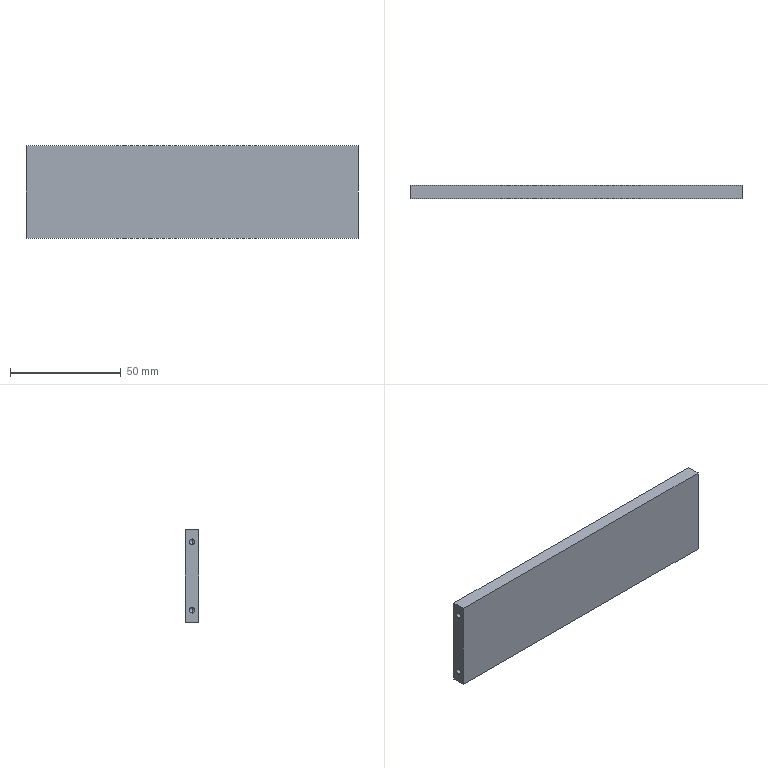Part | SolidWorks | features Cut 2, HoleWzd 2, Extrusion 1 | 1 solid | 22 faces | box 150 x 6 x 42 mm | volume 37648 mm3 | cone 8 | cylinder 8 | plane 6 | commonest cylinder face diameters 2.5 x8
STEP:
#1=CARTESIAN_POINT('',(-66.749,3.,-15.5));
#2=VERTEX_POINT('',#1);
#3=CARTESIAN_POINT('',(-67.5,3.,-14.25));
#4=VERTEX_POINT('',#3);
#5=CARTESIAN_POINT('',(-67.5,3.,-14.25));
#6=DIRECTION('',(-0.515,0.,0.8572));
#7=VECTOR('',#6,1000.);
#8=LINE('',#5,#7);
#9=EDGE_CURVE('',#2,#4,#8,.T.);
#10=ORIENTED_EDGE('',*,*,#9,.F.);
#11=CARTESIAN_POINT('',(-67.5,3.,-16.75));
#12=VERTEX_POINT('',#11);
#13=CARTESIAN_POINT('',(-67.5,3.,-16.75));
#14=DIRECTION('',(-0.515,0.,-0.8572));
#15=VECTOR('',#14,1000.);
#16=LINE('',#13,#15);
#17=EDGE_CURVE('',#2,#12,#16,.T.);
#18=ORIENTED_EDGE('',*,*,#17,.T.);
#19=CARTESIAN_POINT('',(-67.5,3.,-15.5));
#20=DIRECTION('',(-1.,0.,0.));
#21=DIRECTION('',(0.,0.,1.));
#22=AXIS2_PLACEMENT_3D('',#19,#20,#21);
#23=CIRCLE('',#22,1.25);
#24=EDGE_CURVE('',#12,#4,#23,.T.);
#25=ORIENTED_EDGE('',*,*,#24,.T.);
#26=EDGE_LOOP('',(#10,#18,#25));
#27=FACE_OUTER_BOUND('',#26,.T.);
#28=CARTESIAN_POINT('',(-67.5,3.,-15.5));
#29=DIRECTION('',(-1.,0.,0.));
#30=DIRECTION('',(0.,0.,1.));
#31=AXIS2_PLACEMENT_3D('',#28,#29,#30);
#32=CONICAL_SURFACE('',#31,1.25,1.03);
#33=ADVANCED_FACE('',(#27),#32,.F.);
#34=CARTESIAN_POINT('',(-66.749,3.,15.5));
#35=VERTEX_POINT('',#34);
#36=CARTESIAN_POINT('',(-67.5,3.,16.75));
#37=VERTEX_POINT('',#36);
#38=CARTESIAN_POINT('',(-67.5,3.,16.75));
#39=DIRECTION('',(-0.515,0.,0.8572));
#40=VECTOR('',#39,1000.);
#41=LINE('',#38,#40);
#42=EDGE_CURVE('',#35,#37,#41,.T.);
#43=ORIENTED_EDGE('',*,*,#42,.F.);
#44=CARTESIAN_POINT('',(-67.5,3.,14.25));
#45=VERTEX_POINT('',#44);
#46=CARTESIAN_POINT('',(-67.5,3.,14.25));
#47=DIRECTION('',(-0.515,0.,-0.8572));
#48=VECTOR('',#47,1000.);
#49=LINE('',#46,#48);
#50=EDGE_CURVE('',#35,#45,#49,.T.);
#51=ORIENTED_EDGE('',*,*,#50,.T.);
#52=CARTESIAN_POINT('',(-67.5,3.,15.5));
#53=DIRECTION('',(-1.,0.,0.));
#54=DIRECTION('',(0.,0.,1.));
#55=AXIS2_PLACEMENT_3D('',#52,#53,#54);
#56=CIRCLE('',#55,1.25);
#57=EDGE_CURVE('',#45,#37,#56,.T.);
#58=ORIENTED_EDGE('',*,*,#57,.T.);
#59=EDGE_LOOP('',(#43,#51,#58));
#60=FACE_OUTER_BOUND('',#59,.T.);
#61=CARTESIAN_POINT('',(-67.5,3.,15.5));
#62=DIRECTION('',(-1.,0.,0.));
#63=DIRECTION('',(0.,0.,1.));
#64=AXIS2_PLACEMENT_3D('',#61,#62,#63);
#65=CONICAL_SURFACE('',#64,1.25,1.03);
#66=ADVANCED_FACE('',(#60),#65,.F.);
#67=CARTESIAN_POINT('',(66.749,3.,15.5));
#68=VERTEX_POINT('',#67);
#69=CARTESIAN_POINT('',(67.5,3.,14.25));
#70=VERTEX_POINT('',#69);
#71=CARTESIAN_POINT('',(67.5,3.,14.25));
#72=DIRECTION('',(0.515,0.,-0.8572));
#73=VECTOR('',#72,1000.);
#74=LINE('',#71,#73);
#75=EDGE_CURVE('',#68,#70,#74,.T.);
#76=ORIENTED_EDGE('',*,*,#75,.F.);
#77=CARTESIAN_POINT('',(67.5,3.,16.75));
#78=VERTEX_POINT('',#77);
#79=CARTESIAN_POINT('',(67.5,3.,16.75));
#80=DIRECTION('',(0.515,0.,0.8572));
#81=VECTOR('',#80,1000.);
#82=LINE('',#79,#81);
#83=EDGE_CURVE('',#68,#78,#82,.T.);
#84=ORIENTED_EDGE('',*,*,#83,.T.);
#85=CARTESIAN_POINT('',(67.5,3.,15.5));
#86=DIRECTION('',(1.,0.,0.));
#87=DIRECTION('',(0.,0.,-1.));
#88=AXIS2_PLACEMENT_3D('',#85,#86,#87);
#89=CIRCLE('',#88,1.25);
#90=EDGE_CURVE('',#78,#70,#89,.T.);
#91=ORIENTED_EDGE('',*,*,#90,.T.);
#92=EDGE_LOOP('',(#76,#84,#91));
#93=FACE_OUTER_BOUND('',#92,.T.);
#94=CARTESIAN_POINT('',(67.5,3.,15.5));
#95=DIRECTION('',(1.,0.,0.));
#96=DIRECTION('',(0.,0.,-1.));
#97=AXIS2_PLACEMENT_3D('',#94,#95,#96);
#98=CONICAL_SURFACE('',#97,1.25,1.03);
#99=ADVANCED_FACE('',(#93),#98,.F.);
#100=CARTESIAN_POINT('',(66.749,3.,-15.5));
#101=VERTEX_POINT('',#100);
#102=CARTESIAN_POINT('',(67.5,3.,-16.75));
#103=VERTEX_POINT('',#102);
#104=CARTESIAN_POINT('',(67.5,3.,-16.75));
#105=DIRECTION('',(0.515,0.,-0.8572));
#106=VECTOR('',#105,1000.);
#107=LINE('',#104,#106);
#108=EDGE_CURVE('',#101,#103,#107,.T.);
#109=ORIENTED_EDGE('',*,*,#108,.F.);
#110=CARTESIAN_POINT('',(67.5,3.,-14.25));
#111=VERTEX_POINT('',#110);
#112=CARTESIAN_POINT('',(67.5,3.,-14.25));
#113=DIRECTION('',(0.515,0.,0.8572));
#114=VECTOR('',#113,1000.);
#115=LINE('',#112,#114);
#116=EDGE_CURVE('',#101,#111,#115,.T.);
#117=ORIENTED_EDGE('',*,*,#116,.T.);
#118=CARTESIAN_POINT('',(67.5,3.,-15.5));
#119=DIRECTION('',(1.,0.,0.));
#120=DIRECTION('',(0.,0.,-1.));
#121=AXIS2_PLACEMENT_3D('',#118,#119,#120);
#122=CIRCLE('',#121,1.25);
#123=EDGE_CURVE('',#111,#103,#122,.T.);
#124=ORIENTED_EDGE('',*,*,#123,.T.);
#125=EDGE_LOOP('',(#109,#117,#124));
#126=FACE_OUTER_BOUND('',#125,.T.);
#127=CARTESIAN_POINT('',(67.5,3.,-15.5));
#128=DIRECTION('',(1.,0.,0.));
#129=DIRECTION('',(0.,0.,-1.));
#130=AXIS2_PLACEMENT_3D('',#127,#128,#129);
#131=CONICAL_SURFACE('',#130,1.25,1.03);
#132=ADVANCED_FACE('',(#126),#131,.F.);
#133=ORIENTED_EDGE('',*,*,#24,.F.);
#134=CARTESIAN_POINT('',(-75.,3.,-16.75));
#135=VERTEX_POINT('',#134);
#136=CARTESIAN_POINT('',(-70.,3.,-16.75));
#137=DIRECTION('',(-1.,0.,0.));
#138=VECTOR('',#137,1000.);
#139=LINE('',#136,#138);
#140=EDGE_CURVE('',#12,#135,#139,.T.);
#141=ORIENTED_EDGE('',*,*,#140,.T.);
#142=CARTESIAN_POINT('',(-75.,3.,-14.25));
#143=VERTEX_POINT('',#142);
#144=CARTESIAN_POINT('',(-75.,3.,-15.5));
#145=DIRECTION('',(-1.,0.,0.));
#146=DIRECTION('',(0.,0.,1.));
#147=AXIS2_PLACEMENT_3D('',#144,#145,#146);
#148=CIRCLE('',#147,1.25);
#149=EDGE_CURVE('',#135,#143,#148,.T.);
#150=ORIENTED_EDGE('',*,*,#149,.T.);
#151=CARTESIAN_POINT('',(-70.,3.,-14.25));
#152=DIRECTION('',(-1.,0.,0.));
#153=VECTOR('',#152,1000.);
#154=LINE('',#151,#153);
#155=EDGE_CURVE('',#4,#143,#154,.T.);
#156=ORIENTED_EDGE('',*,*,#155,.F.);
#157=EDGE_LOOP('',(#133,#141,#150,#156));
#158=FACE_OUTER_BOUND('',#157,.T.);
#159=CARTESIAN_POINT('',(-70.,3.,-15.5));
#160=DIRECTION('',(-1.,0.,0.));
#161=DIRECTION('',(0.,0.,1.));
#162=AXIS2_PLACEMENT_3D('',#159,#160,#161);
#163=CYLINDRICAL_SURFACE('',#162,1.25);
#164=ADVANCED_FACE('',(#158),#163,.F.);
#165=ORIENTED_EDGE('',*,*,#57,.F.);
#166=CARTESIAN_POINT('',(-75.,3.,14.25));
#167=VERTEX_POINT('',#166);
#168=CARTESIAN_POINT('',(-70.,3.,14.25));
#169=DIRECTION('',(-1.,0.,0.));
#170=VECTOR('',#169,1000.);
#171=LINE('',#168,#170);
#172=EDGE_CURVE('',#45,#167,#171,.T.);
#173=ORIENTED_EDGE('',*,*,#172,.T.);
#174=CARTESIAN_POINT('',(-75.,3.,16.75));
#175=VERTEX_POINT('',#174);
#176=CARTESIAN_POINT('',(-75.,3.,15.5));
#177=DIRECTION('',(-1.,0.,0.));
#178=DIRECTION('',(0.,0.,1.));
#179=AXIS2_PLACEMENT_3D('',#176,#177,#178);
#180=CIRCLE('',#179,1.25);
#181=EDGE_CURVE('',#167,#175,#180,.T.);
#182=ORIENTED_EDGE('',*,*,#181,.T.);
#183=CARTESIAN_POINT('',(-70.,3.,16.75));
#184=DIRECTION('',(-1.,0.,0.));
#185=VECTOR('',#184,1000.);
#186=LINE('',#183,#185);
#187=EDGE_CURVE('',#37,#175,#186,.T.);
#188=ORIENTED_EDGE('',*,*,#187,.F.);
#189=EDGE_LOOP('',(#165,#173,#182,#188));
#190=FACE_OUTER_BOUND('',#189,.T.);
#191=CARTESIAN_POINT('',(-70.,3.,15.5));
#192=DIRECTION('',(-1.,0.,0.));
#193=DIRECTION('',(0.,0.,1.));
#194=AXIS2_PLACEMENT_3D('',#191,#192,#193);
#195=CYLINDRICAL_SURFACE('',#194,1.25);
#196=ADVANCED_FACE('',(#190),#195,.F.);
#197=ORIENTED_EDGE('',*,*,#123,.F.);
#198=CARTESIAN_POINT('',(75.,3.,-14.25));
#199=VERTEX_POINT('',#198);
#200=CARTESIAN_POINT('',(70.,3.,-14.25));
#201=DIRECTION('',(1.,0.,0.));
#202=VECTOR('',#201,1000.);
#203=LINE('',#200,#202);
#204=EDGE_CURVE('',#111,#199,#203,.T.);
#205=ORIENTED_EDGE('',*,*,#204,.T.);
#206=CARTESIAN_POINT('',(75.,3.,-16.75));
#207=VERTEX_POINT('',#206);
#208=CARTESIAN_POINT('',(75.,3.,-15.5));
#209=DIRECTION('',(1.,0.,0.));
#210=DIRECTION('',(0.,0.,-1.));
#211=AXIS2_PLACEMENT_3D('',#208,#209,#210);
#212=CIRCLE('',#211,1.25);
#213=EDGE_CURVE('',#199,#207,#212,.T.);
#214=ORIENTED_EDGE('',*,*,#213,.T.);
#215=CARTESIAN_POINT('',(70.,3.,-16.75));
#216=DIRECTION('',(1.,0.,0.));
#217=VECTOR('',#216,1000.);
#218=LINE('',#215,#217);
#219=EDGE_CURVE('',#103,#207,#218,.T.);
#220=ORIENTED_EDGE('',*,*,#219,.F.);
#221=EDGE_LOOP('',(#197,#205,#214,#220));
#222=FACE_OUTER_BOUND('',#221,.T.);
#223=CARTESIAN_POINT('',(70.,3.,-15.5));
#224=DIRECTION('',(1.,0.,0.));
#225=DIRECTION('',(0.,0.,-1.));
#226=AXIS2_PLACEMENT_3D('',#223,#224,#225);
#227=CYLINDRICAL_SURFACE('',#226,1.25);
#228=ADVANCED_FACE('',(#222),#227,.F.);
#229=ORIENTED_EDGE('',*,*,#90,.F.);
#230=CARTESIAN_POINT('',(75.,3.,16.75));
#231=VERTEX_POINT('',#230);
#232=CARTESIAN_POINT('',(70.,3.,16.75));
#233=DIRECTION('',(1.,0.,0.));
#234=VECTOR('',#233,1000.);
#235=LINE('',#232,#234);
#236=EDGE_CURVE('',#78,#231,#235,.T.);
#237=ORIENTED_EDGE('',*,*,#236,.T.);
#238=CARTESIAN_POINT('',(75.,3.,14.25));
#239=VERTEX_POINT('',#238);
#240=CARTESIAN_POINT('',(75.,3.,15.5));
#241=DIRECTION('',(1.,0.,0.));
#242=DIRECTION('',(0.,0.,-1.));
#243=AXIS2_PLACEMENT_3D('',#240,#241,#242);
#244=CIRCLE('',#243,1.25);
#245=EDGE_CURVE('',#231,#239,#244,.T.);
#246=ORIENTED_EDGE('',*,*,#245,.T.);
#247=CARTESIAN_POINT('',(70.,3.,14.25));
#248=DIRECTION('',(1.,0.,0.));
#249=VECTOR('',#248,1000.);
#250=LINE('',#247,#249);
#251=EDGE_CURVE('',#70,#239,#250,.T.);
#252=ORIENTED_EDGE('',*,*,#251,.F.);
#253=EDGE_LOOP('',(#229,#237,#246,#252));
#254=FACE_OUTER_BOUND('',#253,.T.);
#255=CARTESIAN_POINT('',(70.,3.,15.5));
#256=DIRECTION('',(1.,0.,0.));
#257=DIRECTION('',(0.,0.,-1.));
#258=AXIS2_PLACEMENT_3D('',#255,#256,#257);
#259=CYLINDRICAL_SURFACE('',#258,1.25);
#260=ADVANCED_FACE('',(#254),#259,.F.);
#261=CARTESIAN_POINT('',(75.,3.,-15.5));
#262=DIRECTION('',(1.,0.,0.));
#263=DIRECTION('',(0.,0.,-1.));
#264=AXIS2_PLACEMENT_3D('',#261,#262,#263);
#265=CIRCLE('',#264,1.25);
#266=EDGE_CURVE('',#207,#199,#265,.T.);
#267=ORIENTED_EDGE('',*,*,#266,.F.);
#268=ORIENTED_EDGE('',*,*,#213,.F.);
#269=EDGE_LOOP('',(#267,#268));
#270=FACE_BOUND('',#269,.T.);
#271=CARTESIAN_POINT('',(75.,3.,15.5));
#272=DIRECTION('',(1.,0.,0.));
#273=DIRECTION('',(0.,0.,-1.));
#274=AXIS2_PLACEMENT_3D('',#271,#272,#273);
#275=CIRCLE('',#274,1.25);
#276=EDGE_CURVE('',#239,#231,#275,.T.);
#277=ORIENTED_EDGE('',*,*,#276,.F.);
#278=ORIENTED_EDGE('',*,*,#245,.F.);
#279=EDGE_LOOP('',(#277,#278));
#280=FACE_BOUND('',#279,.T.);
#281=CARTESIAN_POINT('',(75.,0.,21.));
#282=VERTEX_POINT('',#281);
#283=CARTESIAN_POINT('',(75.,0.,-21.));
#284=VERTEX_POINT('',#283);
#285=CARTESIAN_POINT('',(75.,0.,-21.));
#286=DIRECTION('',(0.,0.,-1.));
#287=VECTOR('',#286,1000.);
#288=LINE('',#285,#287);
#289=EDGE_CURVE('',#282,#284,#288,.T.);
#290=ORIENTED_EDGE('',*,*,#289,.T.);
#291=CARTESIAN_POINT('',(75.,6.,-21.));
#292=VERTEX_POINT('',#291);
#293=CARTESIAN_POINT('',(75.,6.,-21.));
#294=DIRECTION('',(0.,-1.,0.));
#295=VECTOR('',#294,1000.);
#296=LINE('',#293,#295);
#297=EDGE_CURVE('',#292,#284,#296,.T.);
#298=ORIENTED_EDGE('',*,*,#297,.F.);
#299=CARTESIAN_POINT('',(75.,6.,21.));
#300=VERTEX_POINT('',#299);
#301=CARTESIAN_POINT('',(75.,6.,-21.));
#302=DIRECTION('',(0.,0.,-1.));
#303=VECTOR('',#302,1000.);
#304=LINE('',#301,#303);
#305=EDGE_CURVE('',#300,#292,#304,.T.);
#306=ORIENTED_EDGE('',*,*,#305,.F.);
#307=CARTESIAN_POINT('',(75.,6.,21.));
#308=DIRECTION('',(0.,-1.,0.));
#309=VECTOR('',#308,1000.);
#310=LINE('',#307,#309);
#311=EDGE_CURVE('',#300,#282,#310,.T.);
#312=ORIENTED_EDGE('',*,*,#311,.T.);
#313=EDGE_LOOP('',(#290,#298,#306,#312));
#314=FACE_OUTER_BOUND('',#313,.T.);
#315=CARTESIAN_POINT('',(75.,6.,-21.));
#316=DIRECTION('',(-1.,0.,0.));
#317=DIRECTION('',(0.,0.,1.));
#318=AXIS2_PLACEMENT_3D('',#315,#316,#317);
#319=PLANE('',#318);
#320=ADVANCED_FACE('',(#270,#280,#314),#319,.F.);
#321=CARTESIAN_POINT('',(-75.,0.,-21.));
#322=VERTEX_POINT('',#321);
#323=CARTESIAN_POINT('',(-75.,0.,-21.));
#324=DIRECTION('',(-1.,0.,0.));
#325=VECTOR('',#324,1000.);
#326=LINE('',#323,#325);
#327=EDGE_CURVE('',#284,#322,#326,.T.);
#328=ORIENTED_EDGE('',*,*,#327,.T.);
#329=CARTESIAN_POINT('',(-75.,6.,-21.));
#330=VERTEX_POINT('',#329);
#331=CARTESIAN_POINT('',(-75.,6.,-21.));
#332=DIRECTION('',(0.,-1.,0.));
#333=VECTOR('',#332,1000.);
#334=LINE('',#331,#333);
#335=EDGE_CURVE('',#330,#322,#334,.T.);
#336=ORIENTED_EDGE('',*,*,#335,.F.);
#337=CARTESIAN_POINT('',(-75.,6.,-21.));
#338=DIRECTION('',(-1.,0.,0.));
#339=VECTOR('',#338,1000.);
#340=LINE('',#337,#339);
#341=EDGE_CURVE('',#292,#330,#340,.T.);
#342=ORIENTED_EDGE('',*,*,#341,.F.);
#343=ORIENTED_EDGE('',*,*,#297,.T.);
#344=EDGE_LOOP('',(#328,#336,#342,#343));
#345=FACE_OUTER_BOUND('',#344,.T.);
#346=CARTESIAN_POINT('',(-75.,6.,-21.));
#347=DIRECTION('',(0.,0.,1.));
#348=DIRECTION('',(1.,0.,0.));
#349=AXIS2_PLACEMENT_3D('',#346,#347,#348);
#350=PLANE('',#349);
#351=ADVANCED_FACE('',(#345),#350,.F.);
#352=CARTESIAN_POINT('',(-75.,3.,-15.5));
#353=DIRECTION('',(-1.,0.,0.));
#354=DIRECTION('',(0.,0.,1.));
#355=AXIS2_PLACEMENT_3D('',#352,#353,#354);
#356=CIRCLE('',#355,1.25);
#357=EDGE_CURVE('',#143,#135,#356,.T.);
#358=ORIENTED_EDGE('',*,*,#357,.F.);
#359=ORIENTED_EDGE('',*,*,#149,.F.);
#360=EDGE_LOOP('',(#358,#359));
#361=FACE_BOUND('',#360,.T.);
#362=CARTESIAN_POINT('',(-75.,3.,15.5));
#363=DIRECTION('',(-1.,0.,0.));
#364=DIRECTION('',(0.,0.,1.));
#365=AXIS2_PLACEMENT_3D('',#362,#363,#364);
#366=CIRCLE('',#365,1.25);
#367=EDGE_CURVE('',#175,#167,#366,.T.);
#368=ORIENTED_EDGE('',*,*,#367,.F.);
#369=ORIENTED_EDGE('',*,*,#181,.F.);
#370=EDGE_LOOP('',(#368,#369));
#371=FACE_BOUND('',#370,.T.);
#372=CARTESIAN_POINT('',(-75.,0.,21.));
#373=VERTEX_POINT('',#372);
#374=CARTESIAN_POINT('',(-75.,0.,-21.));
#375=DIRECTION('',(0.,0.,1.));
#376=VECTOR('',#375,1000.);
#377=LINE('',#374,#376);
#378=EDGE_CURVE('',#322,#373,#377,.T.);
#379=ORIENTED_EDGE('',*,*,#378,.T.);
#380=CARTESIAN_POINT('',(-75.,6.,21.));
#381=VERTEX_POINT('',#380);
#382=CARTESIAN_POINT('',(-75.,6.,21.));
#383=DIRECTION('',(0.,-1.,0.));
#384=VECTOR('',#383,1000.);
#385=LINE('',#382,#384);
#386=EDGE_CURVE('',#381,#373,#385,.T.);
#387=ORIENTED_EDGE('',*,*,#386,.F.);
#388=CARTESIAN_POINT('',(-75.,6.,-21.));
#389=DIRECTION('',(0.,0.,1.));
#390=VECTOR('',#389,1000.);
#391=LINE('',#388,#390);
#392=EDGE_CURVE('',#330,#381,#391,.T.);
#393=ORIENTED_EDGE('',*,*,#392,.F.);
#394=ORIENTED_EDGE('',*,*,#335,.T.);
#395=EDGE_LOOP('',(#379,#387,#393,#394));
#396=FACE_OUTER_BOUND('',#395,.T.);
#397=CARTESIAN_POINT('',(-75.,6.,-21.));
#398=DIRECTION('',(1.,0.,0.));
#399=DIRECTION('',(0.,0.,-1.));
#400=AXIS2_PLACEMENT_3D('',#397,#398,#399);
#401=PLANE('',#400);
#402=ADVANCED_FACE('',(#361,#371,#396),#401,.F.);
#403=CARTESIAN_POINT('',(-75.,0.,21.));
#404=DIRECTION('',(1.,0.,0.));
#405=VECTOR('',#404,1000.);
#406=LINE('',#403,#405);
#407=EDGE_CURVE('',#373,#282,#406,.T.);
#408=ORIENTED_EDGE('',*,*,#407,.T.);
#409=ORIENTED_EDGE('',*,*,#311,.F.);
#410=CARTESIAN_POINT('',(-75.,6.,21.));
#411=DIRECTION('',(1.,0.,0.));
#412=VECTOR('',#411,1000.);
#413=LINE('',#410,#412);
#414=EDGE_CURVE('',#381,#300,#413,.T.);
#415=ORIENTED_EDGE('',*,*,#414,.F.);
#416=ORIENTED_EDGE('',*,*,#386,.T.);
#417=EDGE_LOOP('',(#408,#409,#415,#416));
#418=FACE_OUTER_BOUND('',#417,.T.);
#419=CARTESIAN_POINT('',(-75.,6.,21.));
#420=DIRECTION('',(0.,0.,-1.));
#421=DIRECTION('',(-1.,0.,0.));
#422=AXIS2_PLACEMENT_3D('',#419,#420,#421);
#423=PLANE('',#422);
#424=ADVANCED_FACE('',(#418),#423,.F.);
#425=ORIENTED_EDGE('',*,*,#305,.T.);
#426=ORIENTED_EDGE('',*,*,#341,.T.);
#427=ORIENTED_EDGE('',*,*,#392,.T.);
#428=ORIENTED_EDGE('',*,*,#414,.T.);
#429=EDGE_LOOP('',(#425,#426,#427,#428));
#430=FACE_OUTER_BOUND('',#429,.T.);
#431=CARTESIAN_POINT('',(0.,6.,0.));
#432=DIRECTION('',(0.,1.,0.));
#433=DIRECTION('',(0.,0.,1.));
#434=AXIS2_PLACEMENT_3D('',#431,#432,#433);
#435=PLANE('',#434);
#436=ADVANCED_FACE('',(#430),#435,.T.);
#437=ORIENTED_EDGE('',*,*,#289,.F.);
#438=ORIENTED_EDGE('',*,*,#407,.F.);
#439=ORIENTED_EDGE('',*,*,#378,.F.);
#440=ORIENTED_EDGE('',*,*,#327,.F.);
#441=EDGE_LOOP('',(#437,#438,#439,#440));
#442=FACE_OUTER_BOUND('',#441,.T.);
#443=CARTESIAN_POINT('',(0.,0.,0.));
#444=DIRECTION('',(0.,1.,0.));
#445=DIRECTION('',(0.,0.,1.));
#446=AXIS2_PLACEMENT_3D('',#443,#444,#445);
#447=PLANE('',#446);
#448=ADVANCED_FACE('',(#442),#447,.F.);
#449=ORIENTED_EDGE('',*,*,#236,.F.);
#450=CARTESIAN_POINT('',(67.5,3.,15.5));
#451=DIRECTION('',(1.,0.,0.));
#452=DIRECTION('',(0.,0.,-1.));
#453=AXIS2_PLACEMENT_3D('',#450,#451,#452);
#454=CIRCLE('',#453,1.25);
#455=EDGE_CURVE('',#70,#78,#454,.T.);
#456=ORIENTED_EDGE('',*,*,#455,.F.);
#457=ORIENTED_EDGE('',*,*,#251,.T.);
#458=ORIENTED_EDGE('',*,*,#276,.T.);
#459=EDGE_LOOP('',(#449,#456,#457,#458));
#460=FACE_OUTER_BOUND('',#459,.T.);
#461=CARTESIAN_POINT('',(70.,3.,15.5));
#462=DIRECTION('',(1.,0.,0.));
#463=DIRECTION('',(0.,0.,-1.));
#464=AXIS2_PLACEMENT_3D('',#461,#462,#463);
#465=CYLINDRICAL_SURFACE('',#464,1.25);
#466=ADVANCED_FACE('',(#460),#465,.F.);
#467=ORIENTED_EDGE('',*,*,#204,.F.);
#468=CARTESIAN_POINT('',(67.5,3.,-15.5));
#469=DIRECTION('',(1.,0.,0.));
#470=DIRECTION('',(0.,0.,-1.));
#471=AXIS2_PLACEMENT_3D('',#468,#469,#470);
#472=CIRCLE('',#471,1.25);
#473=EDGE_CURVE('',#103,#111,#472,.T.);
#474=ORIENTED_EDGE('',*,*,#473,.F.);
#475=ORIENTED_EDGE('',*,*,#219,.T.);
#476=ORIENTED_EDGE('',*,*,#266,.T.);
#477=EDGE_LOOP('',(#467,#474,#475,#476));
#478=FACE_OUTER_BOUND('',#477,.T.);
#479=CARTESIAN_POINT('',(70.,3.,-15.5));
#480=DIRECTION('',(1.,0.,0.));
#481=DIRECTION('',(0.,0.,-1.));
#482=AXIS2_PLACEMENT_3D('',#479,#480,#481);
#483=CYLINDRICAL_SURFACE('',#482,1.25);
#484=ADVANCED_FACE('',(#478),#483,.F.);
#485=ORIENTED_EDGE('',*,*,#172,.F.);
#486=CARTESIAN_POINT('',(-67.5,3.,15.5));
#487=DIRECTION('',(-1.,0.,0.));
#488=DIRECTION('',(0.,0.,1.));
#489=AXIS2_PLACEMENT_3D('',#486,#487,#488);
#490=CIRCLE('',#489,1.25);
#491=EDGE_CURVE('',#37,#45,#490,.T.);
#492=ORIENTED_EDGE('',*,*,#491,.F.);
#493=ORIENTED_EDGE('',*,*,#187,.T.);
#494=ORIENTED_EDGE('',*,*,#367,.T.);
#495=EDGE_LOOP('',(#485,#492,#493,#494));
#496=FACE_OUTER_BOUND('',#495,.T.);
#497=CARTESIAN_POINT('',(-70.,3.,15.5));
#498=DIRECTION('',(-1.,0.,0.));
#499=DIRECTION('',(0.,0.,1.));
#500=AXIS2_PLACEMENT_3D('',#497,#498,#499);
#501=CYLINDRICAL_SURFACE('',#500,1.25);
#502=ADVANCED_FACE('',(#496),#501,.F.);
#503=ORIENTED_EDGE('',*,*,#140,.F.);
#504=CARTESIAN_POINT('',(-67.5,3.,-15.5));
#505=DIRECTION('',(-1.,0.,0.));
#506=DIRECTION('',(0.,0.,1.));
#507=AXIS2_PLACEMENT_3D('',#504,#505,#506);
#508=CIRCLE('',#507,1.25);
#509=EDGE_CURVE('',#4,#12,#508,.T.);
#510=ORIENTED_EDGE('',*,*,#509,.F.);
#511=ORIENTED_EDGE('',*,*,#155,.T.);
#512=ORIENTED_EDGE('',*,*,#357,.T.);
#513=EDGE_LOOP('',(#503,#510,#511,#512));
#514=FACE_OUTER_BOUND('',#513,.T.);
#515=CARTESIAN_POINT('',(-70.,3.,-15.5));
#516=DIRECTION('',(-1.,0.,0.));
#517=DIRECTION('',(0.,0.,1.));
#518=AXIS2_PLACEMENT_3D('',#515,#516,#517);
#519=CYLINDRICAL_SURFACE('',#518,1.25);
#520=ADVANCED_FACE('',(#514),#519,.F.);
#521=ORIENTED_EDGE('',*,*,#116,.F.);
#522=ORIENTED_EDGE('',*,*,#108,.T.);
#523=ORIENTED_EDGE('',*,*,#473,.T.);
#524=EDGE_LOOP('',(#521,#522,#523));
#525=FACE_OUTER_BOUND('',#524,.T.);
#526=CARTESIAN_POINT('',(67.5,3.,-15.5));
#527=DIRECTION('',(1.,0.,0.));
#528=DIRECTION('',(0.,0.,-1.));
#529=AXIS2_PLACEMENT_3D('',#526,#527,#528);
#530=CONICAL_SURFACE('',#529,1.25,1.03);
#531=ADVANCED_FACE('',(#525),#530,.F.);
#532=ORIENTED_EDGE('',*,*,#83,.F.);
#533=ORIENTED_EDGE('',*,*,#75,.T.);
#534=ORIENTED_EDGE('',*,*,#455,.T.);
#535=EDGE_LOOP('',(#532,#533,#534));
#536=FACE_OUTER_BOUND('',#535,.T.);
#537=CARTESIAN_POINT('',(67.5,3.,15.5));
#538=DIRECTION('',(1.,0.,0.));
#539=DIRECTION('',(0.,0.,-1.));
#540=AXIS2_PLACEMENT_3D('',#537,#538,#539);
#541=CONICAL_SURFACE('',#540,1.25,1.03);
#542=ADVANCED_FACE('',(#536),#541,.F.);
#543=ORIENTED_EDGE('',*,*,#50,.F.);
#544=ORIENTED_EDGE('',*,*,#42,.T.);
#545=ORIENTED_EDGE('',*,*,#491,.T.);
#546=EDGE_LOOP('',(#543,#544,#545));
#547=FACE_OUTER_BOUND('',#546,.T.);
#548=CARTESIAN_POINT('',(-67.5,3.,15.5));
#549=DIRECTION('',(-1.,0.,0.));
#550=DIRECTION('',(0.,0.,1.));
#551=AXIS2_PLACEMENT_3D('',#548,#549,#550);
#552=CONICAL_SURFACE('',#551,1.25,1.03);
#553=ADVANCED_FACE('',(#547),#552,.F.);
#554=ORIENTED_EDGE('',*,*,#17,.F.);
#555=ORIENTED_EDGE('',*,*,#9,.T.);
#556=ORIENTED_EDGE('',*,*,#509,.T.);
#557=EDGE_LOOP('',(#554,#555,#556));
#558=FACE_OUTER_BOUND('',#557,.T.);
#559=CARTESIAN_POINT('',(-67.5,3.,-15.5));
#560=DIRECTION('',(-1.,0.,0.));
#561=DIRECTION('',(0.,0.,1.));
#562=AXIS2_PLACEMENT_3D('',#559,#560,#561);
#563=CONICAL_SURFACE('',#562,1.25,1.03);
#564=ADVANCED_FACE('',(#558),#563,.F.);
#565=CLOSED_SHELL('',(#33,#66,#99,#132,#164,#196,#228,#260,#320,#351,#402,#424,#436,#448,#466,#484,#502,#520,#531,#542,#553,#564));
#566=MANIFOLD_SOLID_BREP('',#565);
#567=CARTESIAN_POINT('',(0.,0.,0.));
#568=DIRECTION('',(0.,0.,1.));
#569=DIRECTION('',(1.,0.,0.));
#570=AXIS2_PLACEMENT_3D('',#567,#568,#569);
#571=(LENGTH_UNIT()NAMED_UNIT(*)SI_UNIT(.MILLI.,.METRE.));
#572=UNCERTAINTY_MEASURE_WITH_UNIT(LENGTH_MEASURE(0.00001),#571,'','');
#573=(NAMED_UNIT(*)PLANE_ANGLE_UNIT()SI_UNIT($,.RADIAN.));
#574=(NAMED_UNIT(*)SI_UNIT($,.STERADIAN.)SOLID_ANGLE_UNIT());
#575=(GEOMETRIC_REPRESENTATION_CONTEXT(3)GLOBAL_UNCERTAINTY_ASSIGNED_CONTEXT((#572))GLOBAL_UNIT_ASSIGNED_CONTEXT((#571,#573,#574))REPRESENTATION_CONTEXT('',''));
#576=ADVANCED_BREP_SHAPE_REPRESENTATION('',(#566,#570),#575);